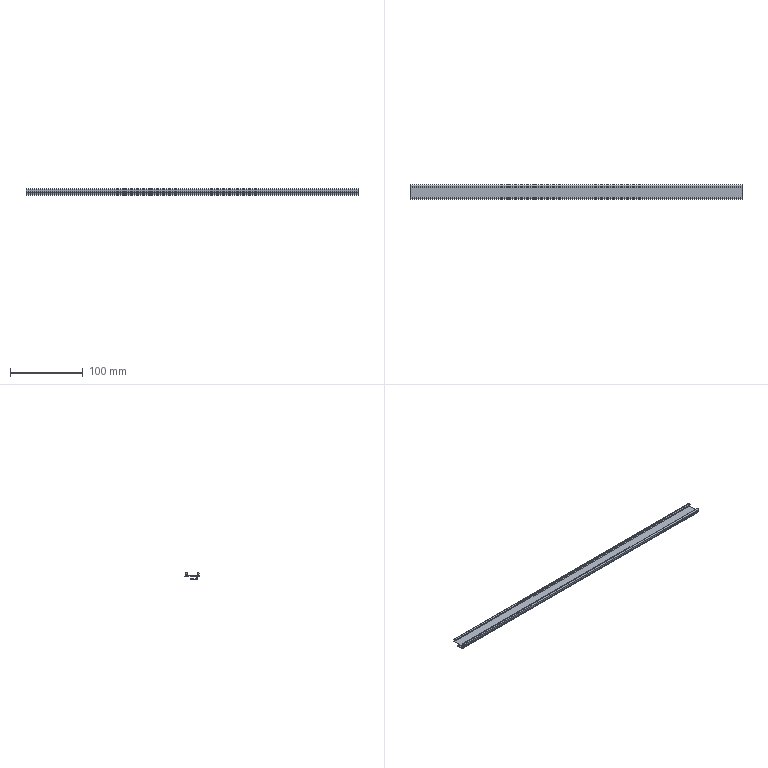Part | SolidWorks | features Extrusion 1 | 1 solid | 38 faces | box 455 x 19.991 x 9 mm | volume 18370 mm3 | cylinder 20 | plane 18 | commonest cylinder face diameters 2 x8 0.5 x5 0.2 x2 3 x2 3.038 x1 3.653 x1
STEP:
#1=CARTESIAN_POINT('',(31.5,952.837,457.965));
#2=VERTEX_POINT('',#1);
#3=CARTESIAN_POINT('',(31.5,952.1,457.));
#4=VERTEX_POINT('',#3);
#5=CARTESIAN_POINT('',(31.5,953.1,457.));
#6=DIRECTION('',(1.,0.,0.));
#7=DIRECTION('',(0.,1.,0.));
#8=AXIS2_PLACEMENT_3D('',#5,#6,#7);
#9=CIRCLE('',#8,1.);
#10=EDGE_CURVE('',#2,#4,#9,.T.);
#11=ORIENTED_EDGE('',*,*,#10,.T.);
#12=CARTESIAN_POINT('',(-423.5,952.1,457.));
#13=VERTEX_POINT('',#12);
#14=CARTESIAN_POINT('',(31.5,952.1,457.));
#15=DIRECTION('',(-1.,0.,0.));
#16=VECTOR('',#15,1000.);
#17=LINE('',#14,#16);
#18=EDGE_CURVE('',#4,#13,#17,.T.);
#19=ORIENTED_EDGE('',*,*,#18,.T.);
#20=CARTESIAN_POINT('',(-423.5,952.837,457.965));
#21=VERTEX_POINT('',#20);
#22=CARTESIAN_POINT('',(-423.5,953.1,457.));
#23=DIRECTION('',(1.,0.,0.));
#24=DIRECTION('',(0.,1.,0.));
#25=AXIS2_PLACEMENT_3D('',#22,#23,#24);
#26=CIRCLE('',#25,1.);
#27=EDGE_CURVE('',#21,#13,#26,.T.);
#28=ORIENTED_EDGE('',*,*,#27,.F.);
#29=CARTESIAN_POINT('',(31.5,952.837,457.965));
#30=DIRECTION('',(-1.,0.,0.));
#31=VECTOR('',#30,1000.);
#32=LINE('',#29,#31);
#33=EDGE_CURVE('',#2,#21,#32,.T.);
#34=ORIENTED_EDGE('',*,*,#33,.F.);
#35=EDGE_LOOP('',(#11,#19,#28,#34));
#36=FACE_OUTER_BOUND('',#35,.T.);
#37=CARTESIAN_POINT('',(31.5,953.1,457.));
#38=DIRECTION('',(-1.,0.,0.));
#39=DIRECTION('',(0.,-1.,0.));
#40=AXIS2_PLACEMENT_3D('',#37,#38,#39);
#41=CYLINDRICAL_SURFACE('',#40,1.);
#42=ADVANCED_FACE('',(#36),#41,.F.);
#43=CARTESIAN_POINT('',(31.5,968.437,458.135));
#44=VERTEX_POINT('',#43);
#45=CARTESIAN_POINT('',(31.5,967.7,459.1));
#46=VERTEX_POINT('',#45);
#47=CARTESIAN_POINT('',(31.5,968.7,459.1));
#48=DIRECTION('',(-1.,0.,0.));
#49=DIRECTION('',(0.,-1.,0.));
#50=AXIS2_PLACEMENT_3D('',#47,#48,#49);
#51=CIRCLE('',#50,1.);
#52=EDGE_CURVE('',#44,#46,#51,.T.);
#53=ORIENTED_EDGE('',*,*,#52,.T.);
#54=CARTESIAN_POINT('',(-423.5,967.7,459.1));
#55=VERTEX_POINT('',#54);
#56=CARTESIAN_POINT('',(31.5,967.7,459.1));
#57=DIRECTION('',(-1.,0.,0.));
#58=VECTOR('',#57,1000.);
#59=LINE('',#56,#58);
#60=EDGE_CURVE('',#46,#55,#59,.T.);
#61=ORIENTED_EDGE('',*,*,#60,.T.);
#62=CARTESIAN_POINT('',(-423.5,968.437,458.135));
#63=VERTEX_POINT('',#62);
#64=CARTESIAN_POINT('',(-423.5,968.7,459.1));
#65=DIRECTION('',(-1.,0.,0.));
#66=DIRECTION('',(0.,-1.,0.));
#67=AXIS2_PLACEMENT_3D('',#64,#65,#66);
#68=CIRCLE('',#67,1.);
#69=EDGE_CURVE('',#63,#55,#68,.T.);
#70=ORIENTED_EDGE('',*,*,#69,.F.);
#71=CARTESIAN_POINT('',(31.5,968.437,458.135));
#72=DIRECTION('',(-1.,0.,0.));
#73=VECTOR('',#72,1000.);
#74=LINE('',#71,#73);
#75=EDGE_CURVE('',#44,#63,#74,.T.);
#76=ORIENTED_EDGE('',*,*,#75,.F.);
#77=EDGE_LOOP('',(#53,#61,#70,#76));
#78=FACE_OUTER_BOUND('',#77,.T.);
#79=CARTESIAN_POINT('',(31.5,968.7,459.1));
#80=DIRECTION('',(-1.,0.,0.));
#81=DIRECTION('',(0.,-1.,0.));
#82=AXIS2_PLACEMENT_3D('',#79,#80,#81);
#83=CYLINDRICAL_SURFACE('',#82,1.);
#84=ADVANCED_FACE('',(#78),#83,.T.);
#85=CARTESIAN_POINT('',(-423.5,955.25,455.2));
#86=VERTEX_POINT('',#85);
#87=CARTESIAN_POINT('',(-423.5,955.,454.95));
#88=VERTEX_POINT('',#87);
#89=CARTESIAN_POINT('',(-423.5,955.25,454.95));
#90=DIRECTION('',(1.,0.,0.));
#91=DIRECTION('',(0.,1.,0.));
#92=AXIS2_PLACEMENT_3D('',#89,#90,#91);
#93=CIRCLE('',#92,0.25);
#94=EDGE_CURVE('',#86,#88,#93,.T.);
#95=ORIENTED_EDGE('',*,*,#94,.F.);
#96=CARTESIAN_POINT('',(31.5,955.25,455.2));
#97=VERTEX_POINT('',#96);
#98=CARTESIAN_POINT('',(31.5,955.25,455.2));
#99=DIRECTION('',(-1.,0.,0.));
#100=VECTOR('',#99,1000.);
#101=LINE('',#98,#100);
#102=EDGE_CURVE('',#97,#86,#101,.T.);
#103=ORIENTED_EDGE('',*,*,#102,.F.);
#104=CARTESIAN_POINT('',(31.5,955.,454.95));
#105=VERTEX_POINT('',#104);
#106=CARTESIAN_POINT('',(31.5,955.25,454.95));
#107=DIRECTION('',(1.,0.,0.));
#108=DIRECTION('',(0.,1.,0.));
#109=AXIS2_PLACEMENT_3D('',#106,#107,#108);
#110=CIRCLE('',#109,0.25);
#111=EDGE_CURVE('',#97,#105,#110,.T.);
#112=ORIENTED_EDGE('',*,*,#111,.T.);
#113=CARTESIAN_POINT('',(31.5,955.,454.95));
#114=DIRECTION('',(-1.,0.,0.));
#115=VECTOR('',#114,1000.);
#116=LINE('',#113,#115);
#117=EDGE_CURVE('',#105,#88,#116,.T.);
#118=ORIENTED_EDGE('',*,*,#117,.T.);
#119=EDGE_LOOP('',(#95,#103,#112,#118));
#120=FACE_OUTER_BOUND('',#119,.T.);
#121=CARTESIAN_POINT('',(31.5,955.25,454.95));
#122=DIRECTION('',(-1.,0.,0.));
#123=DIRECTION('',(0.,-1.,0.));
#124=AXIS2_PLACEMENT_3D('',#121,#122,#123);
#125=CYLINDRICAL_SURFACE('',#124,0.25);
#126=ADVANCED_FACE('',(#120),#125,.F.);
#127=CARTESIAN_POINT('',(-423.5,969.8,455.2));
#128=VERTEX_POINT('',#127);
#129=CARTESIAN_POINT('',(-423.5,969.8,455.2));
#130=DIRECTION('',(0.,-1.,0.));
#131=VECTOR('',#130,1000.);
#132=LINE('',#129,#131);
#133=EDGE_CURVE('',#128,#86,#132,.T.);
#134=ORIENTED_EDGE('',*,*,#133,.F.);
#135=CARTESIAN_POINT('',(31.5,969.8,455.2));
#136=VERTEX_POINT('',#135);
#137=CARTESIAN_POINT('',(31.5,969.8,455.2));
#138=DIRECTION('',(-1.,0.,0.));
#139=VECTOR('',#138,1000.);
#140=LINE('',#137,#139);
#141=EDGE_CURVE('',#136,#128,#140,.T.);
#142=ORIENTED_EDGE('',*,*,#141,.F.);
#143=CARTESIAN_POINT('',(31.5,969.8,455.2));
#144=DIRECTION('',(0.,-1.,0.));
#145=VECTOR('',#144,1000.);
#146=LINE('',#143,#145);
#147=EDGE_CURVE('',#136,#97,#146,.T.);
#148=ORIENTED_EDGE('',*,*,#147,.T.);
#149=ORIENTED_EDGE('',*,*,#102,.T.);
#150=EDGE_LOOP('',(#134,#142,#148,#149));
#151=FACE_OUTER_BOUND('',#150,.T.);
#152=CARTESIAN_POINT('',(31.5,969.8,455.2));
#153=DIRECTION('',(0.,0.,-1.));
#154=DIRECTION('',(0.,1.,0.));
#155=AXIS2_PLACEMENT_3D('',#152,#153,#154);
#156=PLANE('',#155);
#157=ADVANCED_FACE('',(#151),#156,.T.);
#158=CARTESIAN_POINT('',(-423.5,971.025,454.913));
#159=VERTEX_POINT('',#158);
#160=CARTESIAN_POINT('',(-423.5,969.866,452.722));
#161=DIRECTION('',(1.,0.,0.));
#162=DIRECTION('',(0.,1.,0.));
#163=AXIS2_PLACEMENT_3D('',#160,#161,#162);
#164=CIRCLE('',#163,2.479);
#165=EDGE_CURVE('',#159,#128,#164,.T.);
#166=ORIENTED_EDGE('',*,*,#165,.F.);
#167=CARTESIAN_POINT('',(31.5,971.025,454.913));
#168=VERTEX_POINT('',#167);
#169=CARTESIAN_POINT('',(31.5,971.025,454.913));
#170=DIRECTION('',(-1.,0.,0.));
#171=VECTOR('',#170,1000.);
#172=LINE('',#169,#171);
#173=EDGE_CURVE('',#168,#159,#172,.T.);
#174=ORIENTED_EDGE('',*,*,#173,.F.);
#175=CARTESIAN_POINT('',(31.5,969.866,452.722));
#176=DIRECTION('',(1.,0.,0.));
#177=DIRECTION('',(0.,1.,0.));
#178=AXIS2_PLACEMENT_3D('',#175,#176,#177);
#179=CIRCLE('',#178,2.479);
#180=EDGE_CURVE('',#168,#136,#179,.T.);
#181=ORIENTED_EDGE('',*,*,#180,.T.);
#182=ORIENTED_EDGE('',*,*,#141,.T.);
#183=EDGE_LOOP('',(#166,#174,#181,#182));
#184=FACE_OUTER_BOUND('',#183,.T.);
#185=CARTESIAN_POINT('',(31.5,969.866,452.722));
#186=DIRECTION('',(-1.,0.,0.));
#187=DIRECTION('',(0.,-1.,0.));
#188=AXIS2_PLACEMENT_3D('',#185,#186,#187);
#189=CYLINDRICAL_SURFACE('',#188,2.479);
#190=ADVANCED_FACE('',(#184),#189,.F.);
#191=CARTESIAN_POINT('',(-423.5,971.087,454.903));
#192=VERTEX_POINT('',#191);
#193=CARTESIAN_POINT('',(-423.5,971.072,455.002));
#194=DIRECTION('',(-1.,0.,0.));
#195=DIRECTION('',(0.,-1.,0.));
#196=AXIS2_PLACEMENT_3D('',#193,#194,#195);
#197=CIRCLE('',#196,0.1);
#198=EDGE_CURVE('',#192,#159,#197,.T.);
#199=ORIENTED_EDGE('',*,*,#198,.F.);
#200=CARTESIAN_POINT('',(31.5,971.087,454.903));
#201=VERTEX_POINT('',#200);
#202=CARTESIAN_POINT('',(31.5,971.087,454.903));
#203=DIRECTION('',(-1.,0.,0.));
#204=VECTOR('',#203,1000.);
#205=LINE('',#202,#204);
#206=EDGE_CURVE('',#201,#192,#205,.T.);
#207=ORIENTED_EDGE('',*,*,#206,.F.);
#208=CARTESIAN_POINT('',(31.5,971.072,455.002));
#209=DIRECTION('',(-1.,0.,0.));
#210=DIRECTION('',(0.,-1.,0.));
#211=AXIS2_PLACEMENT_3D('',#208,#209,#210);
#212=CIRCLE('',#211,0.1);
#213=EDGE_CURVE('',#201,#168,#212,.T.);
#214=ORIENTED_EDGE('',*,*,#213,.T.);
#215=ORIENTED_EDGE('',*,*,#173,.T.);
#216=EDGE_LOOP('',(#199,#207,#214,#215));
#217=FACE_OUTER_BOUND('',#216,.T.);
#218=CARTESIAN_POINT('',(31.5,971.072,455.002));
#219=DIRECTION('',(-1.,0.,0.));
#220=DIRECTION('',(0.,-1.,0.));
#221=AXIS2_PLACEMENT_3D('',#218,#219,#220);
#222=CYLINDRICAL_SURFACE('',#221,0.1);
#223=ADVANCED_FACE('',(#217),#222,.T.);
#224=CARTESIAN_POINT('',(-423.5,971.285,455.064));
#225=VERTEX_POINT('',#224);
#226=CARTESIAN_POINT('',(-423.5,971.05,455.15));
#227=DIRECTION('',(-1.,0.,0.));
#228=DIRECTION('',(0.,-1.,0.));
#229=AXIS2_PLACEMENT_3D('',#226,#227,#228);
#230=CIRCLE('',#229,0.25);
#231=EDGE_CURVE('',#225,#192,#230,.T.);
#232=ORIENTED_EDGE('',*,*,#231,.F.);
#233=CARTESIAN_POINT('',(31.5,971.285,455.064));
#234=VERTEX_POINT('',#233);
#235=CARTESIAN_POINT('',(31.5,971.285,455.064));
#236=DIRECTION('',(-1.,0.,0.));
#237=VECTOR('',#236,1000.);
#238=LINE('',#235,#237);
#239=EDGE_CURVE('',#234,#225,#238,.T.);
#240=ORIENTED_EDGE('',*,*,#239,.F.);
#241=CARTESIAN_POINT('',(31.5,971.05,455.15));
#242=DIRECTION('',(-1.,0.,0.));
#243=DIRECTION('',(0.,-1.,0.));
#244=AXIS2_PLACEMENT_3D('',#241,#242,#243);
#245=CIRCLE('',#244,0.25);
#246=EDGE_CURVE('',#234,#201,#245,.T.);
#247=ORIENTED_EDGE('',*,*,#246,.T.);
#248=ORIENTED_EDGE('',*,*,#206,.T.);
#249=EDGE_LOOP('',(#232,#240,#247,#248));
#250=FACE_OUTER_BOUND('',#249,.T.);
#251=CARTESIAN_POINT('',(31.5,971.05,455.15));
#252=DIRECTION('',(-1.,0.,0.));
#253=DIRECTION('',(0.,-1.,0.));
#254=AXIS2_PLACEMENT_3D('',#251,#252,#253);
#255=CYLINDRICAL_SURFACE('',#254,0.25);
#256=ADVANCED_FACE('',(#250),#255,.T.);
#257=CARTESIAN_POINT('',(-423.5,971.243,455.183));
#258=VERTEX_POINT('',#257);
#259=CARTESIAN_POINT('',(-423.5,971.191,455.098));
#260=DIRECTION('',(-1.,0.,0.));
#261=DIRECTION('',(0.,-1.,0.));
#262=AXIS2_PLACEMENT_3D('',#259,#260,#261);
#263=CIRCLE('',#262,0.1);
#264=EDGE_CURVE('',#258,#225,#263,.T.);
#265=ORIENTED_EDGE('',*,*,#264,.F.);
#266=CARTESIAN_POINT('',(31.5,971.243,455.183));
#267=VERTEX_POINT('',#266);
#268=CARTESIAN_POINT('',(31.5,971.243,455.183));
#269=DIRECTION('',(-1.,0.,0.));
#270=VECTOR('',#269,1000.);
#271=LINE('',#268,#270);
#272=EDGE_CURVE('',#267,#258,#271,.T.);
#273=ORIENTED_EDGE('',*,*,#272,.F.);
#274=CARTESIAN_POINT('',(31.5,971.191,455.098));
#275=DIRECTION('',(-1.,0.,0.));
#276=DIRECTION('',(0.,-1.,0.));
#277=AXIS2_PLACEMENT_3D('',#274,#275,#276);
#278=CIRCLE('',#277,0.1);
#279=EDGE_CURVE('',#267,#234,#278,.T.);
#280=ORIENTED_EDGE('',*,*,#279,.T.);
#281=ORIENTED_EDGE('',*,*,#239,.T.);
#282=EDGE_LOOP('',(#265,#273,#280,#281));
#283=FACE_OUTER_BOUND('',#282,.T.);
#284=CARTESIAN_POINT('',(31.5,971.191,455.098));
#285=DIRECTION('',(-1.,0.,0.));
#286=DIRECTION('',(0.,-1.,0.));
#287=AXIS2_PLACEMENT_3D('',#284,#285,#286);
#288=CYLINDRICAL_SURFACE('',#287,0.1);
#289=ADVANCED_FACE('',(#283),#288,.T.);
#290=CARTESIAN_POINT('',(-423.5,970.6,456.));
#291=VERTEX_POINT('',#290);
#292=CARTESIAN_POINT('',(-423.5,972.043,456.475));
#293=DIRECTION('',(1.,0.,0.));
#294=DIRECTION('',(0.,1.,0.));
#295=AXIS2_PLACEMENT_3D('',#292,#293,#294);
#296=CIRCLE('',#295,1.519);
#297=EDGE_CURVE('',#291,#258,#296,.T.);
#298=ORIENTED_EDGE('',*,*,#297,.F.);
#299=CARTESIAN_POINT('',(31.5,970.6,456.));
#300=VERTEX_POINT('',#299);
#301=CARTESIAN_POINT('',(31.5,970.6,456.));
#302=DIRECTION('',(-1.,0.,0.));
#303=VECTOR('',#302,1000.);
#304=LINE('',#301,#303);
#305=EDGE_CURVE('',#300,#291,#304,.T.);
#306=ORIENTED_EDGE('',*,*,#305,.F.);
#307=CARTESIAN_POINT('',(31.5,972.043,456.475));
#308=DIRECTION('',(1.,0.,0.));
#309=DIRECTION('',(0.,1.,0.));
#310=AXIS2_PLACEMENT_3D('',#307,#308,#309);
#311=CIRCLE('',#310,1.519);
#312=EDGE_CURVE('',#300,#267,#311,.T.);
#313=ORIENTED_EDGE('',*,*,#312,.T.);
#314=ORIENTED_EDGE('',*,*,#272,.T.);
#315=EDGE_LOOP('',(#298,#306,#313,#314));
#316=FACE_OUTER_BOUND('',#315,.T.);
#317=CARTESIAN_POINT('',(31.5,972.043,456.475));
#318=DIRECTION('',(-1.,0.,0.));
#319=DIRECTION('',(0.,-1.,0.));
#320=AXIS2_PLACEMENT_3D('',#317,#318,#319);
#321=CYLINDRICAL_SURFACE('',#320,1.519);
#322=ADVANCED_FACE('',(#316),#321,.F.);
#323=CARTESIAN_POINT('',(-423.5,970.6,458.6));
#324=VERTEX_POINT('',#323);
#325=CARTESIAN_POINT('',(-423.5,970.6,458.6));
#326=DIRECTION('',(0.,0.,-1.));
#327=VECTOR('',#326,1000.);
#328=LINE('',#325,#327);
#329=EDGE_CURVE('',#324,#291,#328,.T.);
#330=ORIENTED_EDGE('',*,*,#329,.F.);
#331=CARTESIAN_POINT('',(31.5,970.6,458.6));
#332=VERTEX_POINT('',#331);
#333=CARTESIAN_POINT('',(31.5,970.6,458.6));
#334=DIRECTION('',(-1.,0.,0.));
#335=VECTOR('',#334,1000.);
#336=LINE('',#333,#335);
#337=EDGE_CURVE('',#332,#324,#336,.T.);
#338=ORIENTED_EDGE('',*,*,#337,.F.);
#339=CARTESIAN_POINT('',(31.5,970.6,458.6));
#340=DIRECTION('',(0.,0.,-1.));
#341=VECTOR('',#340,1000.);
#342=LINE('',#339,#341);
#343=EDGE_CURVE('',#332,#300,#342,.T.);
#344=ORIENTED_EDGE('',*,*,#343,.T.);
#345=ORIENTED_EDGE('',*,*,#305,.T.);
#346=EDGE_LOOP('',(#330,#338,#344,#345));
#347=FACE_OUTER_BOUND('',#346,.T.);
#348=CARTESIAN_POINT('',(31.5,970.6,458.6));
#349=DIRECTION('',(0.,1.,0.));
#350=DIRECTION('',(-1.,0.,0.));
#351=AXIS2_PLACEMENT_3D('',#348,#349,#350);
#352=PLANE('',#351);
#353=ADVANCED_FACE('',(#347),#352,.T.);
#354=CARTESIAN_POINT('',(-423.5,969.1,460.1));
#355=VERTEX_POINT('',#354);
#356=CARTESIAN_POINT('',(-423.5,969.1,458.6));
#357=DIRECTION('',(-1.,0.,0.));
#358=DIRECTION('',(0.,-1.,0.));
#359=AXIS2_PLACEMENT_3D('',#356,#357,#358);
#360=CIRCLE('',#359,1.5);
#361=EDGE_CURVE('',#355,#324,#360,.T.);
#362=ORIENTED_EDGE('',*,*,#361,.F.);
#363=CARTESIAN_POINT('',(31.5,969.1,460.1));
#364=VERTEX_POINT('',#363);
#365=CARTESIAN_POINT('',(31.5,969.1,460.1));
#366=DIRECTION('',(-1.,0.,0.));
#367=VECTOR('',#366,1000.);
#368=LINE('',#365,#367);
#369=EDGE_CURVE('',#364,#355,#368,.T.);
#370=ORIENTED_EDGE('',*,*,#369,.F.);
#371=CARTESIAN_POINT('',(31.5,969.1,458.6));
#372=DIRECTION('',(-1.,0.,0.));
#373=DIRECTION('',(0.,-1.,0.));
#374=AXIS2_PLACEMENT_3D('',#371,#372,#373);
#375=CIRCLE('',#374,1.5);
#376=EDGE_CURVE('',#364,#332,#375,.T.);
#377=ORIENTED_EDGE('',*,*,#376,.T.);
#378=ORIENTED_EDGE('',*,*,#337,.T.);
#379=EDGE_LOOP('',(#362,#370,#377,#378));
#380=FACE_OUTER_BOUND('',#379,.T.);
#381=CARTESIAN_POINT('',(31.5,969.1,458.6));
#382=DIRECTION('',(-1.,0.,0.));
#383=DIRECTION('',(0.,-1.,0.));
#384=AXIS2_PLACEMENT_3D('',#381,#382,#383);
#385=CYLINDRICAL_SURFACE('',#384,1.5);
#386=ADVANCED_FACE('',(#380),#385,.T.);
#387=CARTESIAN_POINT('',(-423.5,968.7,460.1));
#388=VERTEX_POINT('',#387);
#389=CARTESIAN_POINT('',(-423.5,968.7,460.1));
#390=DIRECTION('',(0.,1.,0.));
#391=VECTOR('',#390,1000.);
#392=LINE('',#389,#391);
#393=EDGE_CURVE('',#388,#355,#392,.T.);
#394=ORIENTED_EDGE('',*,*,#393,.F.);
#395=CARTESIAN_POINT('',(31.5,968.7,460.1));
#396=VERTEX_POINT('',#395);
#397=CARTESIAN_POINT('',(31.5,968.7,460.1));
#398=DIRECTION('',(-1.,0.,0.));
#399=VECTOR('',#398,1000.);
#400=LINE('',#397,#399);
#401=EDGE_CURVE('',#396,#388,#400,.T.);
#402=ORIENTED_EDGE('',*,*,#401,.F.);
#403=CARTESIAN_POINT('',(31.5,968.7,460.1));
#404=DIRECTION('',(0.,1.,0.));
#405=VECTOR('',#404,1000.);
#406=LINE('',#403,#405);
#407=EDGE_CURVE('',#396,#364,#406,.T.);
#408=ORIENTED_EDGE('',*,*,#407,.T.);
#409=ORIENTED_EDGE('',*,*,#369,.T.);
#410=EDGE_LOOP('',(#394,#402,#408,#409));
#411=FACE_OUTER_BOUND('',#410,.T.);
#412=CARTESIAN_POINT('',(31.5,968.7,460.1));
#413=DIRECTION('',(0.,0.,1.));
#414=DIRECTION('',(1.,0.,0.));
#415=AXIS2_PLACEMENT_3D('',#412,#413,#414);
#416=PLANE('',#415);
#417=ADVANCED_FACE('',(#411),#416,.T.);
#418=ORIENTED_EDGE('',*,*,#60,.F.);
#419=CARTESIAN_POINT('',(31.5,968.7,459.1));
#420=DIRECTION('',(-1.,0.,0.));
#421=DIRECTION('',(0.,-1.,0.));
#422=AXIS2_PLACEMENT_3D('',#419,#420,#421);
#423=CIRCLE('',#422,1.);
#424=EDGE_CURVE('',#46,#396,#423,.T.);
#425=ORIENTED_EDGE('',*,*,#424,.T.);
#426=ORIENTED_EDGE('',*,*,#401,.T.);
#427=CARTESIAN_POINT('',(-423.5,968.7,459.1));
#428=DIRECTION('',(-1.,0.,0.));
#429=DIRECTION('',(0.,-1.,0.));
#430=AXIS2_PLACEMENT_3D('',#427,#428,#429);
#431=CIRCLE('',#430,1.);
#432=EDGE_CURVE('',#55,#388,#431,.T.);
#433=ORIENTED_EDGE('',*,*,#432,.F.);
#434=EDGE_LOOP('',(#418,#425,#426,#433));
#435=FACE_OUTER_BOUND('',#434,.T.);
#436=CARTESIAN_POINT('',(31.5,968.7,459.1));
#437=DIRECTION('',(-1.,0.,0.));
#438=DIRECTION('',(0.,-1.,0.));
#439=AXIS2_PLACEMENT_3D('',#436,#437,#438);
#440=CYLINDRICAL_SURFACE('',#439,1.);
#441=ADVANCED_FACE('',(#435),#440,.T.);
#442=CARTESIAN_POINT('',(-423.5,969.063,457.965));
#443=VERTEX_POINT('',#442);
#444=CARTESIAN_POINT('',(-423.5,969.063,457.965));
#445=DIRECTION('',(0.,-0.9649,0.2627));
#446=VECTOR('',#445,1000.);
#447=LINE('',#444,#446);
#448=EDGE_CURVE('',#443,#63,#447,.T.);
#449=ORIENTED_EDGE('',*,*,#448,.F.);
#450=CARTESIAN_POINT('',(31.5,969.063,457.965));
#451=VERTEX_POINT('',#450);
#452=CARTESIAN_POINT('',(31.5,969.063,457.965));
#453=DIRECTION('',(-1.,0.,0.));
#454=VECTOR('',#453,1000.);
#455=LINE('',#452,#454);
#456=EDGE_CURVE('',#451,#443,#455,.T.);
#457=ORIENTED_EDGE('',*,*,#456,.F.);
#458=CARTESIAN_POINT('',(31.5,969.063,457.965));
#459=DIRECTION('',(0.,-0.9649,0.2627));
#460=VECTOR('',#459,1000.);
#461=LINE('',#458,#460);
#462=EDGE_CURVE('',#451,#44,#461,.T.);
#463=ORIENTED_EDGE('',*,*,#462,.T.);
#464=ORIENTED_EDGE('',*,*,#75,.T.);
#465=EDGE_LOOP('',(#449,#457,#463,#464));
#466=FACE_OUTER_BOUND('',#465,.T.);
#467=CARTESIAN_POINT('',(31.5,969.063,457.965));
#468=DIRECTION('',(0.,-0.2627,-0.9649));
#469=DIRECTION('',(0.,0.9649,-0.2627));
#470=AXIS2_PLACEMENT_3D('',#467,#468,#469);
#471=PLANE('',#470);
#472=ADVANCED_FACE('',(#466),#471,.T.);
#473=CARTESIAN_POINT('',(-423.5,968.8,456.));
#474=VERTEX_POINT('',#473);
#475=CARTESIAN_POINT('',(-423.5,968.8,457.));
#476=DIRECTION('',(1.,0.,0.));
#477=DIRECTION('',(0.,1.,0.));
#478=AXIS2_PLACEMENT_3D('',#475,#476,#477);
#479=CIRCLE('',#478,1.);
#480=EDGE_CURVE('',#474,#443,#479,.T.);
#481=ORIENTED_EDGE('',*,*,#480,.F.);
#482=CARTESIAN_POINT('',(31.5,968.8,456.));
#483=VERTEX_POINT('',#482);
#484=CARTESIAN_POINT('',(31.5,968.8,456.));
#485=DIRECTION('',(-1.,0.,0.));
#486=VECTOR('',#485,1000.);
#487=LINE('',#484,#486);
#488=EDGE_CURVE('',#483,#474,#487,.T.);
#489=ORIENTED_EDGE('',*,*,#488,.F.);
#490=CARTESIAN_POINT('',(31.5,968.8,457.));
#491=DIRECTION('',(1.,0.,0.));
#492=DIRECTION('',(0.,1.,0.));
#493=AXIS2_PLACEMENT_3D('',#490,#491,#492);
#494=CIRCLE('',#493,1.);
#495=EDGE_CURVE('',#483,#451,#494,.T.);
#496=ORIENTED_EDGE('',*,*,#495,.T.);
#497=ORIENTED_EDGE('',*,*,#456,.T.);
#498=EDGE_LOOP('',(#481,#489,#496,#497));
#499=FACE_OUTER_BOUND('',#498,.T.);
#500=CARTESIAN_POINT('',(31.5,968.8,457.));
#501=DIRECTION('',(-1.,0.,0.));
#502=DIRECTION('',(0.,-1.,0.));
#503=AXIS2_PLACEMENT_3D('',#500,#501,#502);
#504=CYLINDRICAL_SURFACE('',#503,1.);
#505=ADVANCED_FACE('',(#499),#504,.F.);
#506=CARTESIAN_POINT('',(-423.5,953.1,456.));
#507=VERTEX_POINT('',#506);
#508=CARTESIAN_POINT('',(-423.5,953.1,456.));
#509=DIRECTION('',(0.,1.,0.));
#510=VECTOR('',#509,1000.);
#511=LINE('',#508,#510);
#512=EDGE_CURVE('',#507,#474,#511,.T.);
#513=ORIENTED_EDGE('',*,*,#512,.F.);
#514=CARTESIAN_POINT('',(31.5,953.1,456.));
#515=VERTEX_POINT('',#514);
#516=CARTESIAN_POINT('',(31.5,953.1,456.));
#517=DIRECTION('',(-1.,0.,0.));
#518=VECTOR('',#517,1000.);
#519=LINE('',#516,#518);
#520=EDGE_CURVE('',#515,#507,#519,.T.);
#521=ORIENTED_EDGE('',*,*,#520,.F.);
#522=CARTESIAN_POINT('',(31.5,953.1,456.));
#523=DIRECTION('',(0.,1.,0.));
#524=VECTOR('',#523,1000.);
#525=LINE('',#522,#524);
#526=EDGE_CURVE('',#515,#483,#525,.T.);
#527=ORIENTED_EDGE('',*,*,#526,.T.);
#528=ORIENTED_EDGE('',*,*,#488,.T.);
#529=EDGE_LOOP('',(#513,#521,#527,#528));
#530=FACE_OUTER_BOUND('',#529,.T.);
#531=CARTESIAN_POINT('',(31.5,953.1,456.));
#532=DIRECTION('',(0.,0.,1.));
#533=DIRECTION('',(0.,-1.,0.));
#534=AXIS2_PLACEMENT_3D('',#531,#532,#533);
#535=PLANE('',#534);
#536=ADVANCED_FACE('',(#530),#535,.T.);
#537=ORIENTED_EDGE('',*,*,#18,.F.);
#538=CARTESIAN_POINT('',(31.5,953.1,457.));
#539=DIRECTION('',(1.,0.,0.));
#540=DIRECTION('',(0.,1.,0.));
#541=AXIS2_PLACEMENT_3D('',#538,#539,#540);
#542=CIRCLE('',#541,1.);
#543=EDGE_CURVE('',#4,#515,#542,.T.);
#544=ORIENTED_EDGE('',*,*,#543,.T.);
#545=ORIENTED_EDGE('',*,*,#520,.T.);
#546=CARTESIAN_POINT('',(-423.5,953.1,457.));
#547=DIRECTION('',(1.,0.,0.));
#548=DIRECTION('',(0.,1.,0.));
#549=AXIS2_PLACEMENT_3D('',#546,#547,#548);
#550=CIRCLE('',#549,1.);
#551=EDGE_CURVE('',#13,#507,#550,.T.);
#552=ORIENTED_EDGE('',*,*,#551,.F.);
#553=EDGE_LOOP('',(#537,#544,#545,#552));
#554=FACE_OUTER_BOUND('',#553,.T.);
#555=CARTESIAN_POINT('',(31.5,953.1,457.));
#556=DIRECTION('',(-1.,0.,0.));
#557=DIRECTION('',(0.,-1.,0.));
#558=AXIS2_PLACEMENT_3D('',#555,#556,#557);
#559=CYLINDRICAL_SURFACE('',#558,1.);
#560=ADVANCED_FACE('',(#554),#559,.F.);
#561=CARTESIAN_POINT('',(-423.5,953.463,458.135));
#562=VERTEX_POINT('',#561);
#563=CARTESIAN_POINT('',(-423.5,953.463,458.135));
#564=DIRECTION('',(0.,-0.9649,-0.2627));
#565=VECTOR('',#564,1000.);
#566=LINE('',#563,#565);
#567=EDGE_CURVE('',#562,#21,#566,.T.);
#568=ORIENTED_EDGE('',*,*,#567,.F.);
#569=CARTESIAN_POINT('',(31.5,953.463,458.135));
#570=VERTEX_POINT('',#569);
#571=CARTESIAN_POINT('',(31.5,953.463,458.135));
#572=DIRECTION('',(-1.,0.,0.));
#573=VECTOR('',#572,1000.);
#574=LINE('',#571,#573);
#575=EDGE_CURVE('',#570,#562,#574,.T.);
#576=ORIENTED_EDGE('',*,*,#575,.F.);
#577=CARTESIAN_POINT('',(31.5,953.463,458.135));
#578=DIRECTION('',(0.,-0.9649,-0.2627));
#579=VECTOR('',#578,1000.);
#580=LINE('',#577,#579);
#581=EDGE_CURVE('',#570,#2,#580,.T.);
#582=ORIENTED_EDGE('',*,*,#581,.T.);
#583=ORIENTED_EDGE('',*,*,#33,.T.);
#584=EDGE_LOOP('',(#568,#576,#582,#583));
#585=FACE_OUTER_BOUND('',#584,.T.);
#586=CARTESIAN_POINT('',(31.5,953.463,458.135));
#587=DIRECTION('',(0.,0.2627,-0.9649));
#588=DIRECTION('',(0.,0.9649,0.2627));
#589=AXIS2_PLACEMENT_3D('',#586,#587,#588);
#590=PLANE('',#589);
#591=ADVANCED_FACE('',(#585),#590,.T.);
#592=CARTESIAN_POINT('',(-423.5,953.2,460.1));
#593=VERTEX_POINT('',#592);
#594=CARTESIAN_POINT('',(-423.5,953.2,459.1));
#595=DIRECTION('',(-1.,0.,0.));
#596=DIRECTION('',(0.,-1.,0.));
#597=AXIS2_PLACEMENT_3D('',#594,#595,#596);
#598=CIRCLE('',#597,1.);
#599=EDGE_CURVE('',#593,#562,#598,.T.);
#600=ORIENTED_EDGE('',*,*,#599,.F.);
#601=CARTESIAN_POINT('',(31.5,953.2,460.1));
#602=VERTEX_POINT('',#601);
#603=CARTESIAN_POINT('',(31.5,953.2,460.1));
#604=DIRECTION('',(-1.,0.,0.));
#605=VECTOR('',#604,1000.);
#606=LINE('',#603,#605);
#607=EDGE_CURVE('',#602,#593,#606,.T.);
#608=ORIENTED_EDGE('',*,*,#607,.F.);
#609=CARTESIAN_POINT('',(31.5,953.2,459.1));
#610=DIRECTION('',(-1.,0.,0.));
#611=DIRECTION('',(0.,-1.,0.));
#612=AXIS2_PLACEMENT_3D('',#609,#610,#611);
#613=CIRCLE('',#612,1.);
#614=EDGE_CURVE('',#602,#570,#613,.T.);
#615=ORIENTED_EDGE('',*,*,#614,.T.);
#616=ORIENTED_EDGE('',*,*,#575,.T.);
#617=EDGE_LOOP('',(#600,#608,#615,#616));
#618=FACE_OUTER_BOUND('',#617,.T.);
#619=CARTESIAN_POINT('',(31.5,953.2,459.1));
#620=DIRECTION('',(-1.,0.,0.));
#621=DIRECTION('',(0.,-1.,0.));
#622=AXIS2_PLACEMENT_3D('',#619,#620,#621);
#623=CYLINDRICAL_SURFACE('',#622,1.);
#624=ADVANCED_FACE('',(#618),#623,.T.);
#625=CARTESIAN_POINT('',(-423.5,952.8,460.1));
#626=VERTEX_POINT('',#625);
#627=CARTESIAN_POINT('',(-423.5,952.8,460.1));
#628=DIRECTION('',(0.,1.,0.));
#629=VECTOR('',#628,1000.);
#630=LINE('',#627,#629);
#631=EDGE_CURVE('',#626,#593,#630,.T.);
#632=ORIENTED_EDGE('',*,*,#631,.F.);
#633=CARTESIAN_POINT('',(31.5,952.8,460.1));
#634=VERTEX_POINT('',#633);
#635=CARTESIAN_POINT('',(31.5,952.8,460.1));
#636=DIRECTION('',(-1.,0.,0.));
#637=VECTOR('',#636,1000.);
#638=LINE('',#635,#637);
#639=EDGE_CURVE('',#634,#626,#638,.T.);
#640=ORIENTED_EDGE('',*,*,#639,.F.);
#641=CARTESIAN_POINT('',(31.5,952.8,460.1));
#642=DIRECTION('',(0.,1.,0.));
#643=VECTOR('',#642,1000.);
#644=LINE('',#641,#643);
#645=EDGE_CURVE('',#634,#602,#644,.T.);
#646=ORIENTED_EDGE('',*,*,#645,.T.);
#647=ORIENTED_EDGE('',*,*,#607,.T.);
#648=EDGE_LOOP('',(#632,#640,#646,#647));
#649=FACE_OUTER_BOUND('',#648,.T.);
#650=CARTESIAN_POINT('',(31.5,952.8,460.1));
#651=DIRECTION('',(0.,0.,1.));
#652=DIRECTION('',(1.,0.,0.));
#653=AXIS2_PLACEMENT_3D('',#650,#651,#652);
#654=PLANE('',#653);
#655=ADVANCED_FACE('',(#649),#654,.T.);
#656=CARTESIAN_POINT('',(-423.5,951.3,458.6));
#657=VERTEX_POINT('',#656);
#658=CARTESIAN_POINT('',(-423.5,952.8,458.6));
#659=DIRECTION('',(-1.,0.,0.));
#660=DIRECTION('',(0.,-1.,0.));
#661=AXIS2_PLACEMENT_3D('',#658,#659,#660);
#662=CIRCLE('',#661,1.5);
#663=EDGE_CURVE('',#657,#626,#662,.T.);
#664=ORIENTED_EDGE('',*,*,#663,.F.);
#665=CARTESIAN_POINT('',(31.5,951.3,458.6));
#666=VERTEX_POINT('',#665);
#667=CARTESIAN_POINT('',(31.5,951.3,458.6));
#668=DIRECTION('',(-1.,0.,0.));
#669=VECTOR('',#668,1000.);
#670=LINE('',#667,#669);
#671=EDGE_CURVE('',#666,#657,#670,.T.);
#672=ORIENTED_EDGE('',*,*,#671,.F.);
#673=CARTESIAN_POINT('',(31.5,952.8,458.6));
#674=DIRECTION('',(-1.,0.,0.));
#675=DIRECTION('',(0.,-1.,0.));
#676=AXIS2_PLACEMENT_3D('',#673,#674,#675);
#677=CIRCLE('',#676,1.5);
#678=EDGE_CURVE('',#666,#634,#677,.T.);
#679=ORIENTED_EDGE('',*,*,#678,.T.);
#680=ORIENTED_EDGE('',*,*,#639,.T.);
#681=EDGE_LOOP('',(#664,#672,#679,#680));
#682=FACE_OUTER_BOUND('',#681,.T.);
#683=CARTESIAN_POINT('',(31.5,952.8,458.6));
#684=DIRECTION('',(-1.,0.,0.));
#685=DIRECTION('',(0.,-1.,0.));
#686=AXIS2_PLACEMENT_3D('',#683,#684,#685);
#687=CYLINDRICAL_SURFACE('',#686,1.5);
#688=ADVANCED_FACE('',(#682),#687,.T.);
#689=CARTESIAN_POINT('',(-423.5,951.3,456.2));
#690=VERTEX_POINT('',#689);
#691=CARTESIAN_POINT('',(-423.5,951.3,456.2));
#692=DIRECTION('',(0.,0.,1.));
#693=VECTOR('',#692,1000.);
#694=LINE('',#691,#693);
#695=EDGE_CURVE('',#690,#657,#694,.T.);
#696=ORIENTED_EDGE('',*,*,#695,.F.);
#697=CARTESIAN_POINT('',(31.5,951.3,456.2));
#698=VERTEX_POINT('',#697);
#699=CARTESIAN_POINT('',(31.5,951.3,456.2));
#700=DIRECTION('',(-1.,0.,0.));
#701=VECTOR('',#700,1000.);
#702=LINE('',#699,#701);
#703=EDGE_CURVE('',#698,#690,#702,.T.);
#704=ORIENTED_EDGE('',*,*,#703,.F.);
#705=CARTESIAN_POINT('',(31.5,951.3,456.2));
#706=DIRECTION('',(0.,0.,1.));
#707=VECTOR('',#706,1000.);
#708=LINE('',#705,#707);
#709=EDGE_CURVE('',#698,#666,#708,.T.);
#710=ORIENTED_EDGE('',*,*,#709,.T.);
#711=ORIENTED_EDGE('',*,*,#671,.T.);
#712=EDGE_LOOP('',(#696,#704,#710,#711));
#713=FACE_OUTER_BOUND('',#712,.T.);
#714=CARTESIAN_POINT('',(31.5,951.3,456.2));
#715=DIRECTION('',(0.,-1.,0.));
#716=DIRECTION('',(0.,0.,-1.));
#717=AXIS2_PLACEMENT_3D('',#714,#715,#716);
#718=PLANE('',#717);
#719=ADVANCED_FACE('',(#713),#718,.T.);
#720=CARTESIAN_POINT('',(-423.5,952.3,455.2));
#721=VERTEX_POINT('',#720);
#722=CARTESIAN_POINT('',(-423.5,952.3,456.2));
#723=DIRECTION('',(-1.,0.,0.));
#724=DIRECTION('',(0.,-1.,0.));
#725=AXIS2_PLACEMENT_3D('',#722,#723,#724);
#726=CIRCLE('',#725,1.);
#727=EDGE_CURVE('',#721,#690,#726,.T.);
#728=ORIENTED_EDGE('',*,*,#727,.F.);
#729=CARTESIAN_POINT('',(31.5,952.3,455.2));
#730=VERTEX_POINT('',#729);
#731=CARTESIAN_POINT('',(31.5,952.3,455.2));
#732=DIRECTION('',(-1.,0.,0.));
#733=VECTOR('',#732,1000.);
#734=LINE('',#731,#733);
#735=EDGE_CURVE('',#730,#721,#734,.T.);
#736=ORIENTED_EDGE('',*,*,#735,.F.);
#737=CARTESIAN_POINT('',(31.5,952.3,456.2));
#738=DIRECTION('',(-1.,0.,0.));
#739=DIRECTION('',(0.,-1.,0.));
#740=AXIS2_PLACEMENT_3D('',#737,#738,#739);
#741=CIRCLE('',#740,1.);
#742=EDGE_CURVE('',#730,#698,#741,.T.);
#743=ORIENTED_EDGE('',*,*,#742,.T.);
#744=ORIENTED_EDGE('',*,*,#703,.T.);
#745=EDGE_LOOP('',(#728,#736,#743,#744));
#746=FACE_OUTER_BOUND('',#745,.T.);
#747=CARTESIAN_POINT('',(31.5,952.3,456.2));
#748=DIRECTION('',(-1.,0.,0.));
#749=DIRECTION('',(0.,-1.,0.));
#750=AXIS2_PLACEMENT_3D('',#747,#748,#749);
#751=CYLINDRICAL_SURFACE('',#750,1.);
#752=ADVANCED_FACE('',(#746),#751,.T.);
#753=CARTESIAN_POINT('',(-423.5,952.373,455.2));
#754=VERTEX_POINT('',#753);
#755=CARTESIAN_POINT('',(-423.5,952.373,455.2));
#756=DIRECTION('',(0.,-1.,0.));
#757=VECTOR('',#756,1000.);
#758=LINE('',#755,#757);
#759=EDGE_CURVE('',#754,#721,#758,.T.);
#760=ORIENTED_EDGE('',*,*,#759,.F.);
#761=CARTESIAN_POINT('',(31.5,952.373,455.2));
#762=VERTEX_POINT('',#761);
#763=CARTESIAN_POINT('',(31.5,952.373,455.2));
#764=DIRECTION('',(-1.,0.,0.));
#765=VECTOR('',#764,1000.);
#766=LINE('',#763,#765);
#767=EDGE_CURVE('',#762,#754,#766,.T.);
#768=ORIENTED_EDGE('',*,*,#767,.F.);
#769=CARTESIAN_POINT('',(31.5,952.373,455.2));
#770=DIRECTION('',(0.,-1.,0.));
#771=VECTOR('',#770,1000.);
#772=LINE('',#769,#771);
#773=EDGE_CURVE('',#762,#730,#772,.T.);
#774=ORIENTED_EDGE('',*,*,#773,.T.);
#775=ORIENTED_EDGE('',*,*,#735,.T.);
#776=EDGE_LOOP('',(#760,#768,#774,#775));
#777=FACE_OUTER_BOUND('',#776,.T.);
#778=CARTESIAN_POINT('',(31.5,952.373,455.2));
#779=DIRECTION('',(0.,0.,-1.));
#780=DIRECTION('',(-1.,0.,0.));
#781=AXIS2_PLACEMENT_3D('',#778,#779,#780);
#782=PLANE('',#781);
#783=ADVANCED_FACE('',(#777),#782,.T.);
#784=CARTESIAN_POINT('',(-423.5,954.2,453.373));
#785=VERTEX_POINT('',#784);
#786=CARTESIAN_POINT('',(-423.5,952.373,453.373));
#787=DIRECTION('',(1.,0.,0.));
#788=DIRECTION('',(0.,1.,0.));
#789=AXIS2_PLACEMENT_3D('',#786,#787,#788);
#790=CIRCLE('',#789,1.827);
#791=EDGE_CURVE('',#785,#754,#790,.T.);
#792=ORIENTED_EDGE('',*,*,#791,.F.);
#793=CARTESIAN_POINT('',(31.5,954.2,453.373));
#794=VERTEX_POINT('',#793);
#795=CARTESIAN_POINT('',(31.5,954.2,453.373));
#796=DIRECTION('',(-1.,0.,0.));
#797=VECTOR('',#796,1000.);
#798=LINE('',#795,#797);
#799=EDGE_CURVE('',#794,#785,#798,.T.);
#800=ORIENTED_EDGE('',*,*,#799,.F.);
#801=CARTESIAN_POINT('',(31.5,952.373,453.373));
#802=DIRECTION('',(1.,0.,0.));
#803=DIRECTION('',(0.,1.,0.));
#804=AXIS2_PLACEMENT_3D('',#801,#802,#803);
#805=CIRCLE('',#804,1.827);
#806=EDGE_CURVE('',#794,#762,#805,.T.);
#807=ORIENTED_EDGE('',*,*,#806,.T.);
#808=ORIENTED_EDGE('',*,*,#767,.T.);
#809=EDGE_LOOP('',(#792,#800,#807,#808));
#810=FACE_OUTER_BOUND('',#809,.T.);
#811=CARTESIAN_POINT('',(31.5,952.373,453.373));
#812=DIRECTION('',(-1.,0.,0.));
#813=DIRECTION('',(0.,-1.,0.));
#814=AXIS2_PLACEMENT_3D('',#811,#812,#813);
#815=CYLINDRICAL_SURFACE('',#814,1.827);
#816=ADVANCED_FACE('',(#810),#815,.F.);
#817=CARTESIAN_POINT('',(-423.5,954.2,452.1));
#818=VERTEX_POINT('',#817);
#819=CARTESIAN_POINT('',(-423.5,954.2,452.1));
#820=DIRECTION('',(0.,0.,1.));
#821=VECTOR('',#820,1000.);
#822=LINE('',#819,#821);
#823=EDGE_CURVE('',#818,#785,#822,.T.);
#824=ORIENTED_EDGE('',*,*,#823,.F.);
#825=CARTESIAN_POINT('',(31.5,954.2,452.1));
#826=VERTEX_POINT('',#825);
#827=CARTESIAN_POINT('',(31.5,954.2,452.1));
#828=DIRECTION('',(-1.,0.,0.));
#829=VECTOR('',#828,1000.);
#830=LINE('',#827,#829);
#831=EDGE_CURVE('',#826,#818,#830,.T.);
#832=ORIENTED_EDGE('',*,*,#831,.F.);
#833=CARTESIAN_POINT('',(31.5,954.2,452.1));
#834=DIRECTION('',(0.,0.,1.));
#835=VECTOR('',#834,1000.);
#836=LINE('',#833,#835);
#837=EDGE_CURVE('',#826,#794,#836,.T.);
#838=ORIENTED_EDGE('',*,*,#837,.T.);
#839=ORIENTED_EDGE('',*,*,#799,.T.);
#840=EDGE_LOOP('',(#824,#832,#838,#839));
#841=FACE_OUTER_BOUND('',#840,.T.);
#842=CARTESIAN_POINT('',(31.5,954.2,452.1));
#843=DIRECTION('',(0.,-1.,0.));
#844=DIRECTION('',(0.,0.,-1.));
#845=AXIS2_PLACEMENT_3D('',#842,#843,#844);
#846=PLANE('',#845);
#847=ADVANCED_FACE('',(#841),#846,.T.);
#848=CARTESIAN_POINT('',(-423.5,955.2,451.1));
#849=VERTEX_POINT('',#848);
#850=CARTESIAN_POINT('',(-423.5,955.2,452.1));
#851=DIRECTION('',(-1.,0.,0.));
#852=DIRECTION('',(0.,-1.,0.));
#853=AXIS2_PLACEMENT_3D('',#850,#851,#852);
#854=CIRCLE('',#853,1.);
#855=EDGE_CURVE('',#849,#818,#854,.T.);
#856=ORIENTED_EDGE('',*,*,#855,.F.);
#857=CARTESIAN_POINT('',(31.5,955.2,451.1));
#858=VERTEX_POINT('',#857);
#859=CARTESIAN_POINT('',(31.5,955.2,451.1));
#860=DIRECTION('',(-1.,0.,0.));
#861=VECTOR('',#860,1000.);
#862=LINE('',#859,#861);
#863=EDGE_CURVE('',#858,#849,#862,.T.);
#864=ORIENTED_EDGE('',*,*,#863,.F.);
#865=CARTESIAN_POINT('',(31.5,955.2,452.1));
#866=DIRECTION('',(-1.,0.,0.));
#867=DIRECTION('',(0.,-1.,0.));
#868=AXIS2_PLACEMENT_3D('',#865,#866,#867);
#869=CIRCLE('',#868,1.);
#870=EDGE_CURVE('',#858,#826,#869,.T.);
#871=ORIENTED_EDGE('',*,*,#870,.T.);
#872=ORIENTED_EDGE('',*,*,#831,.T.);
#873=EDGE_LOOP('',(#856,#864,#871,#872));
#874=FACE_OUTER_BOUND('',#873,.T.);
#875=CARTESIAN_POINT('',(31.5,955.2,452.1));
#876=DIRECTION('',(-1.,0.,0.));
#877=DIRECTION('',(0.,-1.,0.));
#878=AXIS2_PLACEMENT_3D('',#875,#876,#877);
#879=CYLINDRICAL_SURFACE('',#878,1.);
#880=ADVANCED_FACE('',(#874),#879,.T.);
#881=CARTESIAN_POINT('',(-423.5,962.45,451.1));
#882=VERTEX_POINT('',#881);
#883=CARTESIAN_POINT('',(-423.5,962.45,451.1));
#884=DIRECTION('',(0.,-1.,0.));
#885=VECTOR('',#884,1000.);
#886=LINE('',#883,#885);
#887=EDGE_CURVE('',#882,#849,#886,.T.);
#888=ORIENTED_EDGE('',*,*,#887,.F.);
#889=CARTESIAN_POINT('',(31.5,962.45,451.1));
#890=VERTEX_POINT('',#889);
#891=CARTESIAN_POINT('',(31.5,962.45,451.1));
#892=DIRECTION('',(-1.,0.,0.));
#893=VECTOR('',#892,1000.);
#894=LINE('',#891,#893);
#895=EDGE_CURVE('',#890,#882,#894,.T.);
#896=ORIENTED_EDGE('',*,*,#895,.F.);
#897=CARTESIAN_POINT('',(31.5,962.45,451.1));
#898=DIRECTION('',(0.,-1.,0.));
#899=VECTOR('',#898,1000.);
#900=LINE('',#897,#899);
#901=EDGE_CURVE('',#890,#858,#900,.T.);
#902=ORIENTED_EDGE('',*,*,#901,.T.);
#903=ORIENTED_EDGE('',*,*,#863,.T.);
#904=EDGE_LOOP('',(#888,#896,#902,#903));
#905=FACE_OUTER_BOUND('',#904,.T.);
#906=CARTESIAN_POINT('',(31.5,962.45,451.1));
#907=DIRECTION('',(0.,0.,-1.));
#908=DIRECTION('',(-1.,0.,0.));
#909=AXIS2_PLACEMENT_3D('',#906,#907,#908);
#910=PLANE('',#909);
#911=ADVANCED_FACE('',(#905),#910,.T.);
#912=CARTESIAN_POINT('',(-423.5,962.7,451.35));
#913=VERTEX_POINT('',#912);
#914=CARTESIAN_POINT('',(-423.5,962.45,451.35));
#915=DIRECTION('',(-1.,0.,0.));
#916=DIRECTION('',(0.,-1.,0.));
#917=AXIS2_PLACEMENT_3D('',#914,#915,#916);
#918=CIRCLE('',#917,0.25);
#919=EDGE_CURVE('',#913,#882,#918,.T.);
#920=ORIENTED_EDGE('',*,*,#919,.F.);
#921=CARTESIAN_POINT('',(31.5,962.7,451.35));
#922=VERTEX_POINT('',#921);
#923=CARTESIAN_POINT('',(31.5,962.7,451.35));
#924=DIRECTION('',(-1.,0.,0.));
#925=VECTOR('',#924,1000.);
#926=LINE('',#923,#925);
#927=EDGE_CURVE('',#922,#913,#926,.T.);
#928=ORIENTED_EDGE('',*,*,#927,.F.);
#929=CARTESIAN_POINT('',(31.5,962.45,451.35));
#930=DIRECTION('',(-1.,0.,0.));
#931=DIRECTION('',(0.,-1.,0.));
#932=AXIS2_PLACEMENT_3D('',#929,#930,#931);
#933=CIRCLE('',#932,0.25);
#934=EDGE_CURVE('',#922,#890,#933,.T.);
#935=ORIENTED_EDGE('',*,*,#934,.T.);
#936=ORIENTED_EDGE('',*,*,#895,.T.);
#937=EDGE_LOOP('',(#920,#928,#935,#936));
#938=FACE_OUTER_BOUND('',#937,.T.);
#939=CARTESIAN_POINT('',(31.5,962.45,451.35));
#940=DIRECTION('',(-1.,0.,0.));
#941=DIRECTION('',(0.,-1.,0.));
#942=AXIS2_PLACEMENT_3D('',#939,#940,#941);
#943=CYLINDRICAL_SURFACE('',#942,0.25);
#944=ADVANCED_FACE('',(#938),#943,.T.);
#945=CARTESIAN_POINT('',(-423.5,962.7,452.45));
#946=VERTEX_POINT('',#945);
#947=CARTESIAN_POINT('',(-423.5,962.7,452.45));
#948=DIRECTION('',(0.,0.,-1.));
#949=VECTOR('',#948,1000.);
#950=LINE('',#947,#949);
#951=EDGE_CURVE('',#946,#913,#950,.T.);
#952=ORIENTED_EDGE('',*,*,#951,.F.);
#953=CARTESIAN_POINT('',(31.5,962.7,452.45));
#954=VERTEX_POINT('',#953);
#955=CARTESIAN_POINT('',(31.5,962.7,452.45));
#956=DIRECTION('',(-1.,0.,0.));
#957=VECTOR('',#956,1000.);
#958=LINE('',#955,#957);
#959=EDGE_CURVE('',#954,#946,#958,.T.);
#960=ORIENTED_EDGE('',*,*,#959,.F.);
#961=CARTESIAN_POINT('',(31.5,962.7,452.45));
#962=DIRECTION('',(0.,0.,-1.));
#963=VECTOR('',#962,1000.);
#964=LINE('',#961,#963);
#965=EDGE_CURVE('',#954,#922,#964,.T.);
#966=ORIENTED_EDGE('',*,*,#965,.T.);
#967=ORIENTED_EDGE('',*,*,#927,.T.);
#968=EDGE_LOOP('',(#952,#960,#966,#967));
#969=FACE_OUTER_BOUND('',#968,.T.);
#970=CARTESIAN_POINT('',(31.5,962.7,452.45));
#971=DIRECTION('',(0.,1.,0.));
#972=DIRECTION('',(-1.,0.,0.));
#973=AXIS2_PLACEMENT_3D('',#970,#971,#972);
#974=PLANE('',#973);
#975=ADVANCED_FACE('',(#969),#974,.T.);
#976=CARTESIAN_POINT('',(-423.5,962.45,452.7));
#977=VERTEX_POINT('',#976);
#978=CARTESIAN_POINT('',(-423.5,962.45,452.45));
#979=DIRECTION('',(-1.,0.,0.));
#980=DIRECTION('',(0.,-1.,0.));
#981=AXIS2_PLACEMENT_3D('',#978,#979,#980);
#982=CIRCLE('',#981,0.25);
#983=EDGE_CURVE('',#977,#946,#982,.T.);
#984=ORIENTED_EDGE('',*,*,#983,.F.);
#985=CARTESIAN_POINT('',(31.5,962.45,452.7));
#986=VERTEX_POINT('',#985);
#987=CARTESIAN_POINT('',(31.5,962.45,452.7));
#988=DIRECTION('',(-1.,0.,0.));
#989=VECTOR('',#988,1000.);
#990=LINE('',#987,#989);
#991=EDGE_CURVE('',#986,#977,#990,.T.);
#992=ORIENTED_EDGE('',*,*,#991,.F.);
#993=CARTESIAN_POINT('',(31.5,962.45,452.45));
#994=DIRECTION('',(-1.,0.,0.));
#995=DIRECTION('',(0.,-1.,0.));
#996=AXIS2_PLACEMENT_3D('',#993,#994,#995);
#997=CIRCLE('',#996,0.25);
#998=EDGE_CURVE('',#986,#954,#997,.T.);
#999=ORIENTED_EDGE('',*,*,#998,.T.);
#1000=ORIENTED_EDGE('',*,*,#959,.T.);
#1001=EDGE_LOOP('',(#984,#992,#999,#1000));
#1002=FACE_OUTER_BOUND('',#1001,.T.);
#1003=CARTESIAN_POINT('',(31.5,962.45,452.45));
#1004=DIRECTION('',(-1.,0.,0.));
#1005=DIRECTION('',(0.,-1.,0.));
#1006=AXIS2_PLACEMENT_3D('',#1003,#1004,#1005);
#1007=CYLINDRICAL_SURFACE('',#1006,0.25);
#1008=ADVANCED_FACE('',(#1002),#1007,.T.);
#1009=CARTESIAN_POINT('',(-423.5,961.9,452.7));
#1010=VERTEX_POINT('',#1009);
#1011=CARTESIAN_POINT('',(-423.5,961.9,452.7));
#1012=DIRECTION('',(0.,1.,0.));
#1013=VECTOR('',#1012,1000.);
#1014=LINE('',#1011,#1013);
#1015=EDGE_CURVE('',#1010,#977,#1014,.T.);
#1016=ORIENTED_EDGE('',*,*,#1015,.F.);
#1017=CARTESIAN_POINT('',(31.5,961.9,452.7));
#1018=VERTEX_POINT('',#1017);
#1019=CARTESIAN_POINT('',(31.5,961.9,452.7));
#1020=DIRECTION('',(-1.,0.,0.));
#1021=VECTOR('',#1020,1000.);
#1022=LINE('',#1019,#1021);
#1023=EDGE_CURVE('',#1018,#1010,#1022,.T.);
#1024=ORIENTED_EDGE('',*,*,#1023,.F.);
#1025=CARTESIAN_POINT('',(31.5,961.9,452.7));
#1026=DIRECTION('',(0.,1.,0.));
#1027=VECTOR('',#1026,1000.);
#1028=LINE('',#1025,#1027);
#1029=EDGE_CURVE('',#1018,#986,#1028,.T.);
#1030=ORIENTED_EDGE('',*,*,#1029,.T.);
#1031=ORIENTED_EDGE('',*,*,#991,.T.);
#1032=EDGE_LOOP('',(#1016,#1024,#1030,#1031));
#1033=FACE_OUTER_BOUND('',#1032,.T.);
#1034=CARTESIAN_POINT('',(31.5,961.9,452.7));
#1035=DIRECTION('',(0.,0.,1.));
#1036=DIRECTION('',(1.,0.,0.));
#1037=AXIS2_PLACEMENT_3D('',#1034,#1035,#1036);
#1038=PLANE('',#1037);
#1039=ADVANCED_FACE('',(#1033),#1038,.T.);
#1040=CARTESIAN_POINT('',(-423.5,961.9,451.9));
#1041=VERTEX_POINT('',#1040);
#1042=CARTESIAN_POINT('',(-423.5,961.9,451.9));
#1043=DIRECTION('',(0.,0.,1.));
#1044=VECTOR('',#1043,1000.);
#1045=LINE('',#1042,#1044);
#1046=EDGE_CURVE('',#1041,#1010,#1045,.T.);
#1047=ORIENTED_EDGE('',*,*,#1046,.F.);
#1048=CARTESIAN_POINT('',(31.5,961.9,451.9));
#1049=VERTEX_POINT('',#1048);
#1050=CARTESIAN_POINT('',(31.5,961.9,451.9));
#1051=DIRECTION('',(-1.,0.,0.));
#1052=VECTOR('',#1051,1000.);
#1053=LINE('',#1050,#1052);
#1054=EDGE_CURVE('',#1049,#1041,#1053,.T.);
#1055=ORIENTED_EDGE('',*,*,#1054,.F.);
#1056=CARTESIAN_POINT('',(31.5,961.9,451.9));
#1057=DIRECTION('',(0.,0.,1.));
#1058=VECTOR('',#1057,1000.);
#1059=LINE('',#1056,#1058);
#1060=EDGE_CURVE('',#1049,#1018,#1059,.T.);
#1061=ORIENTED_EDGE('',*,*,#1060,.T.);
#1062=ORIENTED_EDGE('',*,*,#1023,.T.);
#1063=EDGE_LOOP('',(#1047,#1055,#1061,#1062));
#1064=FACE_OUTER_BOUND('',#1063,.T.);
#1065=CARTESIAN_POINT('',(31.5,961.9,451.9));
#1066=DIRECTION('',(0.,-1.,0.));
#1067=DIRECTION('',(1.,0.,0.));
#1068=AXIS2_PLACEMENT_3D('',#1065,#1066,#1067);
#1069=PLANE('',#1068);
#1070=ADVANCED_FACE('',(#1064),#1069,.T.);
#1071=CARTESIAN_POINT('',(-423.5,955.25,451.9));
#1072=VERTEX_POINT('',#1071);
#1073=CARTESIAN_POINT('',(-423.5,955.25,451.9));
#1074=DIRECTION('',(0.,1.,0.));
#1075=VECTOR('',#1074,1000.);
#1076=LINE('',#1073,#1075);
#1077=EDGE_CURVE('',#1072,#1041,#1076,.T.);
#1078=ORIENTED_EDGE('',*,*,#1077,.F.);
#1079=CARTESIAN_POINT('',(31.5,955.25,451.9));
#1080=VERTEX_POINT('',#1079);
#1081=CARTESIAN_POINT('',(31.5,955.25,451.9));
#1082=DIRECTION('',(-1.,0.,0.));
#1083=VECTOR('',#1082,1000.);
#1084=LINE('',#1081,#1083);
#1085=EDGE_CURVE('',#1080,#1072,#1084,.T.);
#1086=ORIENTED_EDGE('',*,*,#1085,.F.);
#1087=CARTESIAN_POINT('',(31.5,955.25,451.9));
#1088=DIRECTION('',(0.,1.,0.));
#1089=VECTOR('',#1088,1000.);
#1090=LINE('',#1087,#1089);
#1091=EDGE_CURVE('',#1080,#1049,#1090,.T.);
#1092=ORIENTED_EDGE('',*,*,#1091,.T.);
#1093=ORIENTED_EDGE('',*,*,#1054,.T.);
#1094=EDGE_LOOP('',(#1078,#1086,#1092,#1093));
#1095=FACE_OUTER_BOUND('',#1094,.T.);
#1096=CARTESIAN_POINT('',(31.5,955.25,451.9));
#1097=DIRECTION('',(0.,0.,1.));
#1098=DIRECTION('',(0.,-1.,0.));
#1099=AXIS2_PLACEMENT_3D('',#1096,#1097,#1098);
#1100=PLANE('',#1099);
#1101=ADVANCED_FACE('',(#1095),#1100,.T.);
#1102=CARTESIAN_POINT('',(-423.5,955.,452.15));
#1103=VERTEX_POINT('',#1102);
#1104=CARTESIAN_POINT('',(-423.5,955.25,452.15));
#1105=DIRECTION('',(1.,0.,0.));
#1106=DIRECTION('',(0.,1.,0.));
#1107=AXIS2_PLACEMENT_3D('',#1104,#1105,#1106);
#1108=CIRCLE('',#1107,0.25);
#1109=EDGE_CURVE('',#1103,#1072,#1108,.T.);
#1110=ORIENTED_EDGE('',*,*,#1109,.F.);
#1111=CARTESIAN_POINT('',(31.5,955.,452.15));
#1112=VERTEX_POINT('',#1111);
#1113=CARTESIAN_POINT('',(31.5,955.,452.15));
#1114=DIRECTION('',(-1.,0.,0.));
#1115=VECTOR('',#1114,1000.);
#1116=LINE('',#1113,#1115);
#1117=EDGE_CURVE('',#1112,#1103,#1116,.T.);
#1118=ORIENTED_EDGE('',*,*,#1117,.F.);
#1119=CARTESIAN_POINT('',(31.5,955.25,452.15));
#1120=DIRECTION('',(1.,0.,0.));
#1121=DIRECTION('',(0.,1.,0.));
#1122=AXIS2_PLACEMENT_3D('',#1119,#1120,#1121);
#1123=CIRCLE('',#1122,0.25);
#1124=EDGE_CURVE('',#1112,#1080,#1123,.T.);
#1125=ORIENTED_EDGE('',*,*,#1124,.T.);
#1126=ORIENTED_EDGE('',*,*,#1085,.T.);
#1127=EDGE_LOOP('',(#1110,#1118,#1125,#1126));
#1128=FACE_OUTER_BOUND('',#1127,.T.);
#1129=CARTESIAN_POINT('',(31.5,955.25,452.15));
#1130=DIRECTION('',(-1.,0.,0.));
#1131=DIRECTION('',(0.,-1.,0.));
#1132=AXIS2_PLACEMENT_3D('',#1129,#1130,#1131);
#1133=CYLINDRICAL_SURFACE('',#1132,0.25);
#1134=ADVANCED_FACE('',(#1128),#1133,.F.);
#1135=CARTESIAN_POINT('',(-423.5,955.,454.95));
#1136=DIRECTION('',(0.,0.,-1.));
#1137=VECTOR('',#1136,1000.);
#1138=LINE('',#1135,#1137);
#1139=EDGE_CURVE('',#88,#1103,#1138,.T.);
#1140=ORIENTED_EDGE('',*,*,#1139,.F.);
#1141=ORIENTED_EDGE('',*,*,#117,.F.);
#1142=CARTESIAN_POINT('',(31.5,955.,454.95));
#1143=DIRECTION('',(0.,0.,-1.));
#1144=VECTOR('',#1143,1000.);
#1145=LINE('',#1142,#1144);
#1146=EDGE_CURVE('',#105,#1112,#1145,.T.);
#1147=ORIENTED_EDGE('',*,*,#1146,.T.);
#1148=ORIENTED_EDGE('',*,*,#1117,.T.);
#1149=EDGE_LOOP('',(#1140,#1141,#1147,#1148));
#1150=FACE_OUTER_BOUND('',#1149,.T.);
#1151=CARTESIAN_POINT('',(31.5,955.,454.95));
#1152=DIRECTION('',(0.,1.,0.));
#1153=DIRECTION('',(-1.,0.,0.));
#1154=AXIS2_PLACEMENT_3D('',#1151,#1152,#1153);
#1155=PLANE('',#1154);
#1156=ADVANCED_FACE('',(#1150),#1155,.T.);
#1157=ORIENTED_EDGE('',*,*,#111,.F.);
#1158=ORIENTED_EDGE('',*,*,#147,.F.);
#1159=ORIENTED_EDGE('',*,*,#180,.F.);
#1160=ORIENTED_EDGE('',*,*,#213,.F.);
#1161=ORIENTED_EDGE('',*,*,#246,.F.);
#1162=ORIENTED_EDGE('',*,*,#279,.F.);
#1163=ORIENTED_EDGE('',*,*,#312,.F.);
#1164=ORIENTED_EDGE('',*,*,#343,.F.);
#1165=ORIENTED_EDGE('',*,*,#376,.F.);
#1166=ORIENTED_EDGE('',*,*,#407,.F.);
#1167=ORIENTED_EDGE('',*,*,#424,.F.);
#1168=ORIENTED_EDGE('',*,*,#52,.F.);
#1169=ORIENTED_EDGE('',*,*,#462,.F.);
#1170=ORIENTED_EDGE('',*,*,#495,.F.);
#1171=ORIENTED_EDGE('',*,*,#526,.F.);
#1172=ORIENTED_EDGE('',*,*,#543,.F.);
#1173=ORIENTED_EDGE('',*,*,#10,.F.);
#1174=ORIENTED_EDGE('',*,*,#581,.F.);
#1175=ORIENTED_EDGE('',*,*,#614,.F.);
#1176=ORIENTED_EDGE('',*,*,#645,.F.);
#1177=ORIENTED_EDGE('',*,*,#678,.F.);
#1178=ORIENTED_EDGE('',*,*,#709,.F.);
#1179=ORIENTED_EDGE('',*,*,#742,.F.);
#1180=ORIENTED_EDGE('',*,*,#773,.F.);
#1181=ORIENTED_EDGE('',*,*,#806,.F.);
#1182=ORIENTED_EDGE('',*,*,#837,.F.);
#1183=ORIENTED_EDGE('',*,*,#870,.F.);
#1184=ORIENTED_EDGE('',*,*,#901,.F.);
#1185=ORIENTED_EDGE('',*,*,#934,.F.);
#1186=ORIENTED_EDGE('',*,*,#965,.F.);
#1187=ORIENTED_EDGE('',*,*,#998,.F.);
#1188=ORIENTED_EDGE('',*,*,#1029,.F.);
#1189=ORIENTED_EDGE('',*,*,#1060,.F.);
#1190=ORIENTED_EDGE('',*,*,#1091,.F.);
#1191=ORIENTED_EDGE('',*,*,#1124,.F.);
#1192=ORIENTED_EDGE('',*,*,#1146,.F.);
#1193=EDGE_LOOP('',(#1157,#1158,#1159,#1160,#1161,#1162,#1163,#1164,#1165,#1166,#1167,#1168,#1169,#1170,#1171,#1172,#1173,#1174,#1175,#1176,#1177,#1178,#1179,#1180,#1181,#1182,#1183,#1184,#1185,#1186,#1187,#1188,#1189,#1190,#1191,#1192));
#1194=FACE_OUTER_BOUND('',#1193,.T.);
#1195=CARTESIAN_POINT('',(31.5,955.25,454.95));
#1196=DIRECTION('',(1.,0.,0.));
#1197=DIRECTION('',(0.,1.,0.));
#1198=AXIS2_PLACEMENT_3D('',#1195,#1196,#1197);
#1199=PLANE('',#1198);
#1200=ADVANCED_FACE('',(#1194),#1199,.T.);
#1201=ORIENTED_EDGE('',*,*,#94,.T.);
#1202=ORIENTED_EDGE('',*,*,#1139,.T.);
#1203=ORIENTED_EDGE('',*,*,#1109,.T.);
#1204=ORIENTED_EDGE('',*,*,#1077,.T.);
#1205=ORIENTED_EDGE('',*,*,#1046,.T.);
#1206=ORIENTED_EDGE('',*,*,#1015,.T.);
#1207=ORIENTED_EDGE('',*,*,#983,.T.);
#1208=ORIENTED_EDGE('',*,*,#951,.T.);
#1209=ORIENTED_EDGE('',*,*,#919,.T.);
#1210=ORIENTED_EDGE('',*,*,#887,.T.);
#1211=ORIENTED_EDGE('',*,*,#855,.T.);
#1212=ORIENTED_EDGE('',*,*,#823,.T.);
#1213=ORIENTED_EDGE('',*,*,#791,.T.);
#1214=ORIENTED_EDGE('',*,*,#759,.T.);
#1215=ORIENTED_EDGE('',*,*,#727,.T.);
#1216=ORIENTED_EDGE('',*,*,#695,.T.);
#1217=ORIENTED_EDGE('',*,*,#663,.T.);
#1218=ORIENTED_EDGE('',*,*,#631,.T.);
#1219=ORIENTED_EDGE('',*,*,#599,.T.);
#1220=ORIENTED_EDGE('',*,*,#567,.T.);
#1221=ORIENTED_EDGE('',*,*,#27,.T.);
#1222=ORIENTED_EDGE('',*,*,#551,.T.);
#1223=ORIENTED_EDGE('',*,*,#512,.T.);
#1224=ORIENTED_EDGE('',*,*,#480,.T.);
#1225=ORIENTED_EDGE('',*,*,#448,.T.);
#1226=ORIENTED_EDGE('',*,*,#69,.T.);
#1227=ORIENTED_EDGE('',*,*,#432,.T.);
#1228=ORIENTED_EDGE('',*,*,#393,.T.);
#1229=ORIENTED_EDGE('',*,*,#361,.T.);
#1230=ORIENTED_EDGE('',*,*,#329,.T.);
#1231=ORIENTED_EDGE('',*,*,#297,.T.);
#1232=ORIENTED_EDGE('',*,*,#264,.T.);
#1233=ORIENTED_EDGE('',*,*,#231,.T.);
#1234=ORIENTED_EDGE('',*,*,#198,.T.);
#1235=ORIENTED_EDGE('',*,*,#165,.T.);
#1236=ORIENTED_EDGE('',*,*,#133,.T.);
#1237=EDGE_LOOP('',(#1201,#1202,#1203,#1204,#1205,#1206,#1207,#1208,#1209,#1210,#1211,#1212,#1213,#1214,#1215,#1216,#1217,#1218,#1219,#1220,#1221,#1222,#1223,#1224,#1225,#1226,#1227,#1228,#1229,#1230,#1231,#1232,#1233,#1234,#1235,#1236));
#1238=FACE_OUTER_BOUND('',#1237,.T.);
#1239=CARTESIAN_POINT('',(-423.5,955.25,454.95));
#1240=DIRECTION('',(1.,0.,0.));
#1241=DIRECTION('',(0.,1.,0.));
#1242=AXIS2_PLACEMENT_3D('',#1239,#1240,#1241);
#1243=PLANE('',#1242);
#1244=ADVANCED_FACE('',(#1238),#1243,.F.);
#1245=CLOSED_SHELL('',(#42,#84,#126,#157,#190,#223,#256,#289,#322,#353,#386,#417,#441,#472,#505,#536,#560,#591,#624,#655,#688,#719,#752,#783,#816,#847,#880,#911,#944,#975,#1008,#1039,#1070,#1101,#1134,#1156,#1200,#1244));
#1246=MANIFOLD_SOLID_BREP('',#1245);
#1247=CARTESIAN_POINT('',(0.,0.,0.));
#1248=DIRECTION('',(0.,0.,1.));
#1249=DIRECTION('',(1.,0.,0.));
#1250=AXIS2_PLACEMENT_3D('',#1247,#1248,#1249);
#1251=(LENGTH_UNIT()NAMED_UNIT(*)SI_UNIT(.MILLI.,.METRE.));
#1252=UNCERTAINTY_MEASURE_WITH_UNIT(LENGTH_MEASURE(0.00001),#1251,'','');
#1253=(NAMED_UNIT(*)PLANE_ANGLE_UNIT()SI_UNIT($,.RADIAN.));
#1254=(NAMED_UNIT(*)SI_UNIT($,.STERADIAN.)SOLID_ANGLE_UNIT());
#1255=(GEOMETRIC_REPRESENTATION_CONTEXT(3)GLOBAL_UNCERTAINTY_ASSIGNED_CONTEXT((#1252))GLOBAL_UNIT_ASSIGNED_CONTEXT((#1251,#1253,#1254))REPRESENTATION_CONTEXT('',''));
#1256=ADVANCED_BREP_SHAPE_REPRESENTATION('',(#1246,#1250),#1255);